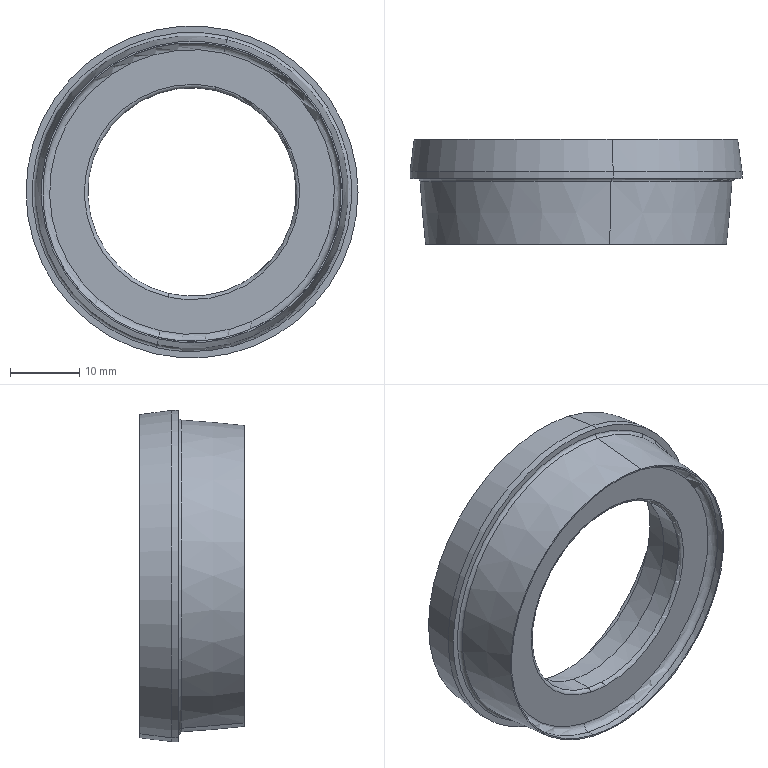Part | SolidWorks | features BaseBody 1 | 1 solid | 37 faces | box 47.8 x 15.1 x 47.8 mm | volume 5914 mm3 | cylinder 12 | torus 12 | plane 7 | cone 6 | commonest cylinder face diameters 30 x2 30.43 x2 35 x2 43 x2 46 x2 47.8 x2
STEP:
#1=CARTESIAN_POINT('',(1958.149,-234.4,875.416));
#2=VERTEX_POINT('',#1);
#3=CARTESIAN_POINT('',(1947.851,-234.4,830.584));
#4=VERTEX_POINT('',#3);
#5=CARTESIAN_POINT('',(1953.,-234.4,853.));
#6=DIRECTION('',(0.,-1.,0.));
#7=DIRECTION('',(0.9746,0.,-0.2239));
#8=AXIS2_PLACEMENT_3D('',#5,#6,#7);
#9=CIRCLE('',#8,23.);
#10=EDGE_CURVE('',#2,#4,#9,.T.);
#11=ORIENTED_EDGE('',*,*,#10,.T.);
#12=CARTESIAN_POINT('',(1947.851,-230.8,830.584));
#13=VERTEX_POINT('',#12);
#14=CARTESIAN_POINT('',(1947.851,-230.045,830.584));
#15=DIRECTION('',(0.,-1.,0.));
#16=VECTOR('',#15,1000.);
#17=LINE('',#14,#16);
#18=EDGE_CURVE('',#13,#4,#17,.T.);
#19=ORIENTED_EDGE('',*,*,#18,.F.);
#20=CARTESIAN_POINT('',(1958.149,-230.8,875.416));
#21=VERTEX_POINT('',#20);
#22=CARTESIAN_POINT('',(1953.,-230.8,853.));
#23=DIRECTION('',(0.,-1.,0.));
#24=DIRECTION('',(0.9746,0.,-0.2239));
#25=AXIS2_PLACEMENT_3D('',#22,#23,#24);
#26=CIRCLE('',#25,23.);
#27=EDGE_CURVE('',#21,#13,#26,.T.);
#28=ORIENTED_EDGE('',*,*,#27,.F.);
#29=CARTESIAN_POINT('',(1958.149,-230.045,875.416));
#30=DIRECTION('',(0.,1.,0.));
#31=VECTOR('',#30,1000.);
#32=LINE('',#29,#31);
#33=EDGE_CURVE('',#2,#21,#32,.T.);
#34=ORIENTED_EDGE('',*,*,#33,.F.);
#35=EDGE_LOOP('',(#11,#19,#28,#34));
#36=FACE_OUTER_BOUND('',#35,.T.);
#37=CARTESIAN_POINT('',(1953.,-230.045,853.));
#38=DIRECTION('',(0.,-1.,0.));
#39=DIRECTION('',(-0.2239,0.,-0.9746));
#40=AXIS2_PLACEMENT_3D('',#37,#38,#39);
#41=CYLINDRICAL_SURFACE('',#40,23.);
#42=ADVANCED_FACE('',(#36),#41,.F.);
#43=CARTESIAN_POINT('',(1957.701,-236.4,873.467));
#44=VERTEX_POINT('',#43);
#45=CARTESIAN_POINT('',(1948.299,-236.4,832.533));
#46=VERTEX_POINT('',#45);
#47=CARTESIAN_POINT('',(1953.,-236.4,853.));
#48=DIRECTION('',(0.,-1.,0.));
#49=DIRECTION('',(0.9746,0.,-0.2239));
#50=AXIS2_PLACEMENT_3D('',#47,#48,#49);
#51=CIRCLE('',#50,21.);
#52=EDGE_CURVE('',#44,#46,#51,.T.);
#53=ORIENTED_EDGE('',*,*,#52,.T.);
#54=CARTESIAN_POINT('',(1948.299,-234.4,832.533));
#55=DIRECTION('',(-0.9746,0.,0.2239));
#56=DIRECTION('',(0.,-1.,0.));
#57=AXIS2_PLACEMENT_3D('',#54,#55,#56);
#58=CIRCLE('',#57,2.);
#59=EDGE_CURVE('',#4,#46,#58,.T.);
#60=ORIENTED_EDGE('',*,*,#59,.F.);
#61=ORIENTED_EDGE('',*,*,#10,.F.);
#62=CARTESIAN_POINT('',(1957.701,-234.4,873.467));
#63=DIRECTION('',(-0.9746,0.,0.2239));
#64=DIRECTION('',(0.,-1.,0.));
#65=AXIS2_PLACEMENT_3D('',#62,#63,#64);
#66=CIRCLE('',#65,2.);
#67=EDGE_CURVE('',#44,#2,#66,.T.);
#68=ORIENTED_EDGE('',*,*,#67,.F.);
#69=EDGE_LOOP('',(#53,#60,#61,#68));
#70=FACE_OUTER_BOUND('',#69,.T.);
#71=CARTESIAN_POINT('',(1953.,-234.4,853.));
#72=DIRECTION('',(0.,-1.,0.));
#73=DIRECTION('',(-0.2239,0.,-0.9746));
#74=AXIS2_PLACEMENT_3D('',#71,#72,#73);
#75=TOROIDAL_SURFACE('',#74,21.,2.);
#76=ADVANCED_FACE('',(#70),#75,.F.);
#77=CARTESIAN_POINT('',(1953.,-230.8,853.));
#78=DIRECTION('',(0.,1.,0.));
#79=DIRECTION('',(0.9746,0.,-0.2239));
#80=AXIS2_PLACEMENT_3D('',#77,#78,#79);
#81=CIRCLE('',#80,23.);
#82=EDGE_CURVE('',#21,#13,#81,.T.);
#83=ORIENTED_EDGE('',*,*,#82,.T.);
#84=ORIENTED_EDGE('',*,*,#18,.T.);
#85=CARTESIAN_POINT('',(1953.,-234.4,853.));
#86=DIRECTION('',(0.,1.,0.));
#87=DIRECTION('',(0.9746,0.,-0.2239));
#88=AXIS2_PLACEMENT_3D('',#85,#86,#87);
#89=CIRCLE('',#88,23.);
#90=EDGE_CURVE('',#2,#4,#89,.T.);
#91=ORIENTED_EDGE('',*,*,#90,.F.);
#92=ORIENTED_EDGE('',*,*,#33,.T.);
#93=EDGE_LOOP('',(#83,#84,#91,#92));
#94=FACE_OUTER_BOUND('',#93,.T.);
#95=CARTESIAN_POINT('',(1953.,-230.045,853.));
#96=DIRECTION('',(0.,-1.,0.));
#97=DIRECTION('',(0.2239,0.,0.9746));
#98=AXIS2_PLACEMENT_3D('',#95,#96,#97);
#99=CYLINDRICAL_SURFACE('',#98,23.);
#100=ADVANCED_FACE('',(#94),#99,.F.);
#101=CARTESIAN_POINT('',(1958.216,-230.8,875.709));
#102=VERTEX_POINT('',#101);
#103=CARTESIAN_POINT('',(1947.784,-230.8,830.291));
#104=VERTEX_POINT('',#103);
#105=CARTESIAN_POINT('',(1953.,-230.8,853.));
#106=DIRECTION('',(0.,-1.,0.));
#107=DIRECTION('',(0.9746,0.,-0.2239));
#108=AXIS2_PLACEMENT_3D('',#105,#106,#107);
#109=CIRCLE('',#108,23.3);
#110=EDGE_CURVE('',#102,#104,#109,.T.);
#111=ORIENTED_EDGE('',*,*,#110,.F.);
#112=CARTESIAN_POINT('',(1958.216,-230.8,875.709));
#113=CARTESIAN_POINT('',(1960.29,-230.8,875.232));
#114=CARTESIAN_POINT('',(1962.31,-230.8,874.519));
#115=CARTESIAN_POINT('',(1964.24,-230.8,873.577));
#116=CARTESIAN_POINT('',(1967.849,-230.8,871.269));
#117=CARTESIAN_POINT('',(1970.846,-230.8,868.208));
#118=CARTESIAN_POINT('',(1972.162,-230.8,866.511));
#119=CARTESIAN_POINT('',(1974.384,-230.8,862.849));
#120=CARTESIAN_POINT('',(1975.723,-230.8,858.779));
#121=CARTESIAN_POINT('',(1976.157,-230.8,856.676));
#122=CARTESIAN_POINT('',(1976.536,-230.8,852.409));
#123=CARTESIAN_POINT('',(1975.943,-230.8,848.166));
#124=CARTESIAN_POINT('',(1975.404,-230.8,846.087));
#125=CARTESIAN_POINT('',(1973.863,-230.8,842.09));
#126=CARTESIAN_POINT('',(1971.46,-230.8,838.544));
#127=CARTESIAN_POINT('',(1970.06,-230.8,836.916));
#128=CARTESIAN_POINT('',(1966.913,-230.8,834.008));
#129=CARTESIAN_POINT('',(1963.192,-230.8,831.885));
#130=CARTESIAN_POINT('',(1961.218,-230.8,831.041));
#131=CARTESIAN_POINT('',(1957.361,-230.8,829.893));
#132=CARTESIAN_POINT('',(1953.354,-230.8,829.59));
#133=CARTESIAN_POINT('',(1951.471,-230.8,829.637));
#134=CARTESIAN_POINT('',(1949.607,-230.8,829.873));
#135=CARTESIAN_POINT('',(1947.784,-230.8,830.291));
#136=B_SPLINE_CURVE_WITH_KNOTS('',5,(#112,#113,#114,#115,#116,#117,#118,#119,#120,#121,#122,#123,#124,#125,#126,#127,#128,#129,#130,#131,#132,#133,#134,#135),.UNSPECIFIED.,.F.,.F.,(6,3,3,3,3,3,3,6),(0.,0.1454,0.2908,0.4361,0.5815,0.7269,0.8723,1.),.UNSPECIFIED.);
#137=EDGE_CURVE('',#102,#104,#136,.T.);
#138=ORIENTED_EDGE('',*,*,#137,.T.);
#139=EDGE_LOOP('',(#111,#138));
#140=FACE_OUTER_BOUND('',#139,.T.);
#141=ORIENTED_EDGE('',*,*,#82,.F.);
#142=ORIENTED_EDGE('',*,*,#27,.T.);
#143=EDGE_LOOP('',(#141,#142));
#144=FACE_BOUND('',#143,.T.);
#145=CARTESIAN_POINT('',(1953.,-230.8,853.));
#146=DIRECTION('',(0.,-1.,0.));
#147=DIRECTION('',(0.2239,0.,0.9746));
#148=AXIS2_PLACEMENT_3D('',#145,#146,#147);
#149=PLANE('',#148);
#150=ADVANCED_FACE('',(#140,#144),#149,.F.);
#151=ORIENTED_EDGE('',*,*,#52,.F.);
#152=CARTESIAN_POINT('',(1957.701,-236.4,873.467));
#153=CARTESIAN_POINT('',(1959.67,-236.4,873.015));
#154=CARTESIAN_POINT('',(1961.585,-236.4,872.326));
#155=CARTESIAN_POINT('',(1963.408,-236.4,871.408));
#156=CARTESIAN_POINT('',(1966.796,-236.4,869.153));
#157=CARTESIAN_POINT('',(1969.553,-236.4,866.159));
#158=CARTESIAN_POINT('',(1970.744,-236.4,864.503));
#159=CARTESIAN_POINT('',(1972.705,-236.4,860.936));
#160=CARTESIAN_POINT('',(1973.764,-236.4,857.006));
#161=CARTESIAN_POINT('',(1974.053,-236.4,854.987));
#162=CARTESIAN_POINT('',(1974.141,-236.4,850.917));
#163=CARTESIAN_POINT('',(1973.261,-236.4,846.944));
#164=CARTESIAN_POINT('',(1972.583,-236.4,845.019));
#165=CARTESIAN_POINT('',(1970.778,-236.4,841.371));
#166=CARTESIAN_POINT('',(1968.159,-236.4,838.256));
#167=CARTESIAN_POINT('',(1966.667,-236.4,836.863));
#168=CARTESIAN_POINT('',(1963.379,-236.4,834.465));
#169=CARTESIAN_POINT('',(1959.616,-236.4,832.915));
#170=CARTESIAN_POINT('',(1957.649,-236.4,832.371));
#171=CARTESIAN_POINT('',(1954.569,-236.4,831.908));
#172=CARTESIAN_POINT('',(1951.473,-236.4,832.014));
#173=CARTESIAN_POINT('',(1950.403,-236.4,832.12));
#174=CARTESIAN_POINT('',(1949.343,-236.4,832.293));
#175=CARTESIAN_POINT('',(1948.299,-236.4,832.533));
#176=B_SPLINE_CURVE_WITH_KNOTS('',5,(#152,#153,#154,#155,#156,#157,#158,#159,#160,#161,#162,#163,#164,#165,#166,#167,#168,#169,#170,#171,#172,#173,#174,#175),.UNSPECIFIED.,.F.,.F.,(6,3,3,3,3,3,3,6),(0.,0.1531,0.3063,0.4594,0.6125,0.7656,0.9188,1.),.UNSPECIFIED.);
#177=EDGE_CURVE('',#44,#46,#176,.T.);
#178=ORIENTED_EDGE('',*,*,#177,.T.);
#179=EDGE_LOOP('',(#151,#178));
#180=FACE_OUTER_BOUND('',#179,.T.);
#181=CARTESIAN_POINT('',(1957.03,-236.4,870.543));
#182=VERTEX_POINT('',#181);
#183=CARTESIAN_POINT('',(1948.97,-236.4,835.457));
#184=VERTEX_POINT('',#183);
#185=CARTESIAN_POINT('',(1957.03,-236.4,870.543));
#186=CARTESIAN_POINT('',(1958.65,-236.4,870.171));
#187=CARTESIAN_POINT('',(1960.228,-236.4,869.612));
#188=CARTESIAN_POINT('',(1961.734,-236.4,868.872));
#189=CARTESIAN_POINT('',(1964.547,-236.4,867.058));
#190=CARTESIAN_POINT('',(1966.873,-236.4,864.65));
#191=CARTESIAN_POINT('',(1967.891,-236.4,863.317));
#192=CARTESIAN_POINT('',(1969.602,-236.4,860.439));
#193=CARTESIAN_POINT('',(1970.611,-236.4,857.247));
#194=CARTESIAN_POINT('',(1970.928,-236.4,855.6));
#195=CARTESIAN_POINT('',(1971.177,-236.4,852.261));
#196=CARTESIAN_POINT('',(1970.658,-236.4,848.954));
#197=CARTESIAN_POINT('',(1970.208,-236.4,847.338));
#198=CARTESIAN_POINT('',(1968.943,-236.4,844.238));
#199=CARTESIAN_POINT('',(1967.005,-236.4,841.509));
#200=CARTESIAN_POINT('',(1965.882,-236.4,840.262));
#201=CARTESIAN_POINT('',(1963.368,-236.4,838.052));
#202=CARTESIAN_POINT('',(1960.417,-236.4,836.472));
#203=CARTESIAN_POINT('',(1958.856,-236.4,835.857));
#204=CARTESIAN_POINT('',(1955.941,-236.4,835.083));
#205=CARTESIAN_POINT('',(1952.936,-236.4,834.926));
#206=CARTESIAN_POINT('',(1951.597,-236.4,834.98));
#207=CARTESIAN_POINT('',(1950.27,-236.4,835.158));
#208=CARTESIAN_POINT('',(1948.97,-236.4,835.457));
#209=B_SPLINE_CURVE_WITH_KNOTS('',5,(#185,#186,#187,#188,#189,#190,#191,#192,#193,#194,#195,#196,#197,#198,#199,#200,#201,#202,#203,#204,#205,#206,#207,#208),.UNSPECIFIED.,.F.,.F.,(6,3,3,3,3,3,3,6),(0.,0.147,0.294,0.4411,0.5881,0.7351,0.8821,1.),.UNSPECIFIED.);
#210=EDGE_CURVE('',#182,#184,#209,.T.);
#211=ORIENTED_EDGE('',*,*,#210,.F.);
#212=CARTESIAN_POINT('',(1953.,-236.4,853.));
#213=DIRECTION('',(0.,-1.,0.));
#214=DIRECTION('',(0.9746,0.,-0.2239));
#215=AXIS2_PLACEMENT_3D('',#212,#213,#214);
#216=CIRCLE('',#215,18.);
#217=EDGE_CURVE('',#182,#184,#216,.T.);
#218=ORIENTED_EDGE('',*,*,#217,.T.);
#219=EDGE_LOOP('',(#211,#218));
#220=FACE_BOUND('',#219,.T.);
#221=CARTESIAN_POINT('',(1953.,-236.4,853.));
#222=DIRECTION('',(0.,-1.,0.));
#223=DIRECTION('',(0.2239,0.,0.9746));
#224=AXIS2_PLACEMENT_3D('',#221,#222,#223);
#225=PLANE('',#224);
#226=ADVANCED_FACE('',(#180,#220),#225,.F.);
#227=ORIENTED_EDGE('',*,*,#90,.T.);
#228=ORIENTED_EDGE('',*,*,#59,.T.);
#229=ORIENTED_EDGE('',*,*,#177,.F.);
#230=ORIENTED_EDGE('',*,*,#67,.T.);
#231=EDGE_LOOP('',(#227,#228,#229,#230));
#232=FACE_OUTER_BOUND('',#231,.T.);
#233=CARTESIAN_POINT('',(1953.,-234.4,853.));
#234=DIRECTION('',(0.,-1.,0.));
#235=DIRECTION('',(0.2239,0.,0.9746));
#236=AXIS2_PLACEMENT_3D('',#233,#234,#235);
#237=TOROIDAL_SURFACE('',#236,21.,2.);
#238=ADVANCED_FACE('',(#232),#237,.F.);
#239=ORIENTED_EDGE('',*,*,#110,.T.);
#240=CARTESIAN_POINT('',(1947.65,-235.4,829.707));
#241=VERTEX_POINT('',#240);
#242=CARTESIAN_POINT('',(-12527.07,-495942.839,-62186.75));
#243=DIRECTION('',(0.02895,0.9916,0.1261));
#244=VECTOR('',#243,1000.);
#245=LINE('',#242,#244);
#246=EDGE_CURVE('',#241,#104,#245,.T.);
#247=ORIENTED_EDGE('',*,*,#246,.F.);
#248=CARTESIAN_POINT('',(1958.35,-235.4,876.293));
#249=VERTEX_POINT('',#248);
#250=CARTESIAN_POINT('',(1953.,-235.4,853.));
#251=DIRECTION('',(0.,-1.,0.));
#252=DIRECTION('',(0.9746,0.,-0.2239));
#253=AXIS2_PLACEMENT_3D('',#250,#251,#252);
#254=CIRCLE('',#253,23.9);
#255=EDGE_CURVE('',#249,#241,#254,.T.);
#256=ORIENTED_EDGE('',*,*,#255,.F.);
#257=CARTESIAN_POINT('',(16433.07,-495942.839,63892.75));
#258=DIRECTION('',(0.02895,-0.9916,0.1261));
#259=VECTOR('',#258,1000.);
#260=LINE('',#257,#259);
#261=EDGE_CURVE('',#102,#249,#260,.T.);
#262=ORIENTED_EDGE('',*,*,#261,.F.);
#263=EDGE_LOOP('',(#239,#247,#256,#262));
#264=FACE_OUTER_BOUND('',#263,.T.);
#265=CARTESIAN_POINT('',(1953.,-233.1,853.));
#266=DIRECTION('',(0.,-1.,0.));
#267=DIRECTION('',(-0.2239,0.,-0.9746));
#268=AXIS2_PLACEMENT_3D('',#265,#266,#267);
#269=CONICAL_SURFACE('',#268,23.6,0.1297);
#270=ADVANCED_FACE('',(#264),#269,.T.);
#271=CARTESIAN_POINT('',(1953.,-235.4,853.));
#272=DIRECTION('',(0.,1.,0.));
#273=DIRECTION('',(0.9746,0.,-0.2239));
#274=AXIS2_PLACEMENT_3D('',#271,#272,#273);
#275=CIRCLE('',#274,23.9);
#276=EDGE_CURVE('',#249,#241,#275,.T.);
#277=ORIENTED_EDGE('',*,*,#276,.T.);
#278=ORIENTED_EDGE('',*,*,#246,.T.);
#279=ORIENTED_EDGE('',*,*,#137,.F.);
#280=ORIENTED_EDGE('',*,*,#261,.T.);
#281=EDGE_LOOP('',(#277,#278,#279,#280));
#282=FACE_OUTER_BOUND('',#281,.T.);
#283=CARTESIAN_POINT('',(1953.,-233.1,853.));
#284=DIRECTION('',(0.,-1.,0.));
#285=DIRECTION('',(0.2239,0.,0.9746));
#286=AXIS2_PLACEMENT_3D('',#283,#284,#285);
#287=CONICAL_SURFACE('',#286,23.6,0.1297);
#288=ADVANCED_FACE('',(#282),#287,.T.);
#289=ORIENTED_EDGE('',*,*,#210,.T.);
#290=CARTESIAN_POINT('',(1949.082,-235.9,835.944));
#291=VERTEX_POINT('',#290);
#292=CARTESIAN_POINT('',(1948.97,-235.9,835.457));
#293=DIRECTION('',(0.9746,0.,-0.2239));
#294=DIRECTION('',(0.,-1.,0.));
#295=AXIS2_PLACEMENT_3D('',#292,#293,#294);
#296=CIRCLE('',#295,0.5);
#297=EDGE_CURVE('',#291,#184,#296,.T.);
#298=ORIENTED_EDGE('',*,*,#297,.F.);
#299=CARTESIAN_POINT('',(1956.918,-235.9,870.056));
#300=VERTEX_POINT('',#299);
#301=CARTESIAN_POINT('',(1953.,-235.9,853.));
#302=DIRECTION('',(0.,1.,0.));
#303=DIRECTION('',(0.9746,0.,-0.2239));
#304=AXIS2_PLACEMENT_3D('',#301,#302,#303);
#305=CIRCLE('',#304,17.5);
#306=EDGE_CURVE('',#300,#291,#305,.T.);
#307=ORIENTED_EDGE('',*,*,#306,.F.);
#308=CARTESIAN_POINT('',(1957.03,-235.9,870.543));
#309=DIRECTION('',(0.9746,0.,-0.2239));
#310=DIRECTION('',(0.,-1.,0.));
#311=AXIS2_PLACEMENT_3D('',#308,#309,#310);
#312=CIRCLE('',#311,0.5);
#313=EDGE_CURVE('',#182,#300,#312,.T.);
#314=ORIENTED_EDGE('',*,*,#313,.F.);
#315=EDGE_LOOP('',(#289,#298,#307,#314));
#316=FACE_OUTER_BOUND('',#315,.T.);
#317=CARTESIAN_POINT('',(1953.,-235.9,853.));
#318=DIRECTION('',(0.,-1.,0.));
#319=DIRECTION('',(0.2239,0.,0.9746));
#320=AXIS2_PLACEMENT_3D('',#317,#318,#319);
#321=TOROIDAL_SURFACE('',#320,18.,0.5);
#322=ADVANCED_FACE('',(#316),#321,.F.);
#323=CARTESIAN_POINT('',(1953.,-235.9,853.));
#324=DIRECTION('',(0.,-1.,0.));
#325=DIRECTION('',(0.9746,0.,-0.2239));
#326=AXIS2_PLACEMENT_3D('',#323,#324,#325);
#327=CIRCLE('',#326,17.5);
#328=EDGE_CURVE('',#300,#291,#327,.T.);
#329=ORIENTED_EDGE('',*,*,#328,.T.);
#330=ORIENTED_EDGE('',*,*,#297,.T.);
#331=ORIENTED_EDGE('',*,*,#217,.F.);
#332=ORIENTED_EDGE('',*,*,#313,.T.);
#333=EDGE_LOOP('',(#329,#330,#331,#332));
#334=FACE_OUTER_BOUND('',#333,.T.);
#335=CARTESIAN_POINT('',(1953.,-235.9,853.));
#336=DIRECTION('',(0.,-1.,0.));
#337=DIRECTION('',(-0.2239,0.,-0.9746));
#338=AXIS2_PLACEMENT_3D('',#335,#336,#337);
#339=TOROIDAL_SURFACE('',#338,18.,0.5);
#340=ADVANCED_FACE('',(#334),#339,.F.);
#341=ORIENTED_EDGE('',*,*,#255,.T.);
#342=CARTESIAN_POINT('',(1947.65,-236.4,829.707));
#343=VERTEX_POINT('',#342);
#344=CARTESIAN_POINT('',(1947.65,-230.045,829.707));
#345=DIRECTION('',(0.,-1.,0.));
#346=VECTOR('',#345,1000.);
#347=LINE('',#344,#346);
#348=EDGE_CURVE('',#241,#343,#347,.T.);
#349=ORIENTED_EDGE('',*,*,#348,.T.);
#350=CARTESIAN_POINT('',(1958.35,-236.4,876.293));
#351=VERTEX_POINT('',#350);
#352=CARTESIAN_POINT('',(1953.,-236.4,853.));
#353=DIRECTION('',(0.,-1.,0.));
#354=DIRECTION('',(0.9746,0.,-0.2239));
#355=AXIS2_PLACEMENT_3D('',#352,#353,#354);
#356=CIRCLE('',#355,23.9);
#357=EDGE_CURVE('',#351,#343,#356,.T.);
#358=ORIENTED_EDGE('',*,*,#357,.F.);
#359=CARTESIAN_POINT('',(1958.35,-230.045,876.293));
#360=DIRECTION('',(0.,1.,0.));
#361=VECTOR('',#360,1000.);
#362=LINE('',#359,#361);
#363=EDGE_CURVE('',#351,#249,#362,.T.);
#364=ORIENTED_EDGE('',*,*,#363,.T.);
#365=EDGE_LOOP('',(#341,#349,#358,#364));
#366=FACE_OUTER_BOUND('',#365,.T.);
#367=CARTESIAN_POINT('',(1953.,-230.045,853.));
#368=DIRECTION('',(0.,-1.,0.));
#369=DIRECTION('',(-0.2239,0.,-0.9746));
#370=AXIS2_PLACEMENT_3D('',#367,#368,#369);
#371=CYLINDRICAL_SURFACE('',#370,23.9);
#372=ADVANCED_FACE('',(#366),#371,.T.);
#373=CARTESIAN_POINT('',(1953.,-236.4,853.));
#374=DIRECTION('',(0.,1.,0.));
#375=DIRECTION('',(0.9746,0.,-0.2239));
#376=AXIS2_PLACEMENT_3D('',#373,#374,#375);
#377=CIRCLE('',#376,23.9);
#378=EDGE_CURVE('',#351,#343,#377,.T.);
#379=ORIENTED_EDGE('',*,*,#378,.T.);
#380=ORIENTED_EDGE('',*,*,#348,.F.);
#381=ORIENTED_EDGE('',*,*,#276,.F.);
#382=ORIENTED_EDGE('',*,*,#363,.F.);
#383=EDGE_LOOP('',(#379,#380,#381,#382));
#384=FACE_OUTER_BOUND('',#383,.T.);
#385=CARTESIAN_POINT('',(1953.,-230.045,853.));
#386=DIRECTION('',(0.,-1.,0.));
#387=DIRECTION('',(0.2239,0.,0.9746));
#388=AXIS2_PLACEMENT_3D('',#385,#386,#387);
#389=CYLINDRICAL_SURFACE('',#388,23.9);
#390=ADVANCED_FACE('',(#384),#389,.T.);
#391=ORIENTED_EDGE('',*,*,#306,.T.);
#392=CARTESIAN_POINT('',(1949.082,-235.4,835.944));
#393=VERTEX_POINT('',#392);
#394=CARTESIAN_POINT('',(1949.082,-230.045,835.944));
#395=DIRECTION('',(0.,1.,0.));
#396=VECTOR('',#395,1000.);
#397=LINE('',#394,#396);
#398=EDGE_CURVE('',#291,#393,#397,.T.);
#399=ORIENTED_EDGE('',*,*,#398,.T.);
#400=CARTESIAN_POINT('',(1956.918,-235.4,870.056));
#401=VERTEX_POINT('',#400);
#402=CARTESIAN_POINT('',(1953.,-235.4,853.));
#403=DIRECTION('',(0.,1.,0.));
#404=DIRECTION('',(0.9746,0.,-0.2239));
#405=AXIS2_PLACEMENT_3D('',#402,#403,#404);
#406=CIRCLE('',#405,17.5);
#407=EDGE_CURVE('',#401,#393,#406,.T.);
#408=ORIENTED_EDGE('',*,*,#407,.F.);
#409=CARTESIAN_POINT('',(1956.918,-230.045,870.056));
#410=DIRECTION('',(0.,-1.,0.));
#411=VECTOR('',#410,1000.);
#412=LINE('',#409,#411);
#413=EDGE_CURVE('',#401,#300,#412,.T.);
#414=ORIENTED_EDGE('',*,*,#413,.T.);
#415=EDGE_LOOP('',(#391,#399,#408,#414));
#416=FACE_OUTER_BOUND('',#415,.T.);
#417=CARTESIAN_POINT('',(1953.,-230.045,853.));
#418=DIRECTION('',(0.,-1.,0.));
#419=DIRECTION('',(0.2239,0.,0.9746));
#420=AXIS2_PLACEMENT_3D('',#417,#418,#419);
#421=CYLINDRICAL_SURFACE('',#420,17.5);
#422=ADVANCED_FACE('',(#416),#421,.T.);
#423=CARTESIAN_POINT('',(1953.,-235.4,853.));
#424=DIRECTION('',(0.,-1.,0.));
#425=DIRECTION('',(0.9746,0.,-0.2239));
#426=AXIS2_PLACEMENT_3D('',#423,#424,#425);
#427=CIRCLE('',#426,17.5);
#428=EDGE_CURVE('',#401,#393,#427,.T.);
#429=ORIENTED_EDGE('',*,*,#428,.T.);
#430=ORIENTED_EDGE('',*,*,#398,.F.);
#431=ORIENTED_EDGE('',*,*,#328,.F.);
#432=ORIENTED_EDGE('',*,*,#413,.F.);
#433=EDGE_LOOP('',(#429,#430,#431,#432));
#434=FACE_OUTER_BOUND('',#433,.T.);
#435=CARTESIAN_POINT('',(1953.,-230.045,853.));
#436=DIRECTION('',(0.,-1.,0.));
#437=DIRECTION('',(-0.2239,0.,-0.9746));
#438=AXIS2_PLACEMENT_3D('',#435,#436,#437);
#439=CYLINDRICAL_SURFACE('',#438,17.5);
#440=ADVANCED_FACE('',(#434),#439,.T.);
#441=ORIENTED_EDGE('',*,*,#378,.F.);
#442=ORIENTED_EDGE('',*,*,#357,.T.);
#443=EDGE_LOOP('',(#441,#442));
#444=FACE_OUTER_BOUND('',#443,.T.);
#445=CARTESIAN_POINT('',(1958.147,-236.4,875.406));
#446=VERTEX_POINT('',#445);
#447=CARTESIAN_POINT('',(1947.853,-236.4,830.594));
#448=VERTEX_POINT('',#447);
#449=CARTESIAN_POINT('',(1953.,-236.4,853.));
#450=DIRECTION('',(0.,-1.,0.));
#451=DIRECTION('',(0.9746,0.,-0.2239));
#452=AXIS2_PLACEMENT_3D('',#449,#450,#451);
#453=CIRCLE('',#452,22.989);
#454=EDGE_CURVE('',#446,#448,#453,.T.);
#455=ORIENTED_EDGE('',*,*,#454,.F.);
#456=CARTESIAN_POINT('',(1958.147,-236.4,875.406));
#457=CARTESIAN_POINT('',(1960.207,-236.4,874.933));
#458=CARTESIAN_POINT('',(1962.213,-236.4,874.222));
#459=CARTESIAN_POINT('',(1964.128,-236.4,873.284));
#460=CARTESIAN_POINT('',(1967.709,-236.4,870.983));
#461=CARTESIAN_POINT('',(1970.674,-236.4,867.93));
#462=CARTESIAN_POINT('',(1971.974,-236.4,866.239));
#463=CARTESIAN_POINT('',(1974.161,-236.4,862.589));
#464=CARTESIAN_POINT('',(1975.464,-236.4,858.537));
#465=CARTESIAN_POINT('',(1975.878,-236.4,856.445));
#466=CARTESIAN_POINT('',(1976.219,-236.4,852.202));
#467=CARTESIAN_POINT('',(1975.588,-236.4,847.993));
#468=CARTESIAN_POINT('',(1975.031,-236.4,845.935));
#469=CARTESIAN_POINT('',(1973.453,-236.4,841.982));
#470=CARTESIAN_POINT('',(1971.02,-236.4,838.49));
#471=CARTESIAN_POINT('',(1969.607,-236.4,836.892));
#472=CARTESIAN_POINT('',(1966.44,-236.4,834.05));
#473=CARTESIAN_POINT('',(1962.71,-236.4,832.));
#474=CARTESIAN_POINT('',(1960.735,-236.4,831.195));
#475=CARTESIAN_POINT('',(1956.978,-236.4,830.149));
#476=CARTESIAN_POINT('',(1953.093,-236.4,829.909));
#477=CARTESIAN_POINT('',(1951.323,-236.4,829.97));
#478=CARTESIAN_POINT('',(1949.569,-236.4,830.2));
#479=CARTESIAN_POINT('',(1947.853,-236.4,830.594));
#480=B_SPLINE_CURVE_WITH_KNOTS('',5,(#456,#457,#458,#459,#460,#461,#462,#463,#464,#465,#466,#467,#468,#469,#470,#471,#472,#473,#474,#475,#476,#477,#478,#479),.UNSPECIFIED.,.F.,.F.,(6,3,3,3,3,3,3,6),(0.,0.1464,0.2927,0.4391,0.5854,0.7318,0.8781,1.),.UNSPECIFIED.);
#481=EDGE_CURVE('',#446,#448,#480,.T.);
#482=ORIENTED_EDGE('',*,*,#481,.T.);
#483=EDGE_LOOP('',(#455,#482));
#484=FACE_BOUND('',#483,.T.);
#485=CARTESIAN_POINT('',(1953.,-236.4,853.));
#486=DIRECTION('',(0.,-1.,0.));
#487=DIRECTION('',(0.2239,0.,0.9746));
#488=AXIS2_PLACEMENT_3D('',#485,#486,#487);
#489=PLANE('',#488);
#490=ADVANCED_FACE('',(#444,#484),#489,.T.);
#491=ORIENTED_EDGE('',*,*,#428,.F.);
#492=ORIENTED_EDGE('',*,*,#407,.T.);
#493=EDGE_LOOP('',(#491,#492));
#494=FACE_OUTER_BOUND('',#493,.T.);
#495=CARTESIAN_POINT('',(1956.851,-235.4,869.763));
#496=VERTEX_POINT('',#495);
#497=CARTESIAN_POINT('',(1949.149,-235.4,836.237));
#498=VERTEX_POINT('',#497);
#499=CARTESIAN_POINT('',(1956.851,-235.4,869.763));
#500=CARTESIAN_POINT('',(1958.435,-235.4,869.4));
#501=CARTESIAN_POINT('',(1959.976,-235.4,868.849));
#502=CARTESIAN_POINT('',(1961.445,-235.4,868.117));
#503=CARTESIAN_POINT('',(1964.181,-235.4,866.321));
#504=CARTESIAN_POINT('',(1966.424,-235.4,863.937));
#505=CARTESIAN_POINT('',(1967.399,-235.4,862.618));
#506=CARTESIAN_POINT('',(1969.019,-235.4,859.773));
#507=CARTESIAN_POINT('',(1969.931,-235.4,856.629));
#508=CARTESIAN_POINT('',(1970.199,-235.4,855.011));
#509=CARTESIAN_POINT('',(1970.346,-235.4,851.74));
#510=CARTESIAN_POINT('',(1969.728,-235.4,848.526));
#511=CARTESIAN_POINT('',(1969.229,-235.4,846.963));
#512=CARTESIAN_POINT('',(1967.873,-235.4,843.984));
#513=CARTESIAN_POINT('',(1965.859,-235.4,841.403));
#514=CARTESIAN_POINT('',(1964.704,-235.4,840.238));
#515=CARTESIAN_POINT('',(1962.14,-235.4,838.203));
#516=CARTESIAN_POINT('',(1959.172,-235.4,836.821));
#517=CARTESIAN_POINT('',(1957.613,-235.4,836.31));
#518=CARTESIAN_POINT('',(1954.967,-235.4,835.778));
#519=CARTESIAN_POINT('',(1952.279,-235.4,835.766));
#520=CARTESIAN_POINT('',(1951.223,-235.4,835.843));
#521=CARTESIAN_POINT('',(1950.177,-235.4,836.));
#522=CARTESIAN_POINT('',(1949.149,-235.4,836.237));
#523=B_SPLINE_CURVE_WITH_KNOTS('',5,(#499,#500,#501,#502,#503,#504,#505,#506,#507,#508,#509,#510,#511,#512,#513,#514,#515,#516,#517,#518,#519,#520,#521,#522),.UNSPECIFIED.,.F.,.F.,(6,3,3,3,3,3,3,6),(0.,0.1504,0.3008,0.4512,0.6016,0.752,0.9024,1.),.UNSPECIFIED.);
#524=EDGE_CURVE('',#496,#498,#523,.T.);
#525=ORIENTED_EDGE('',*,*,#524,.F.);
#526=CARTESIAN_POINT('',(1953.,-235.4,853.));
#527=DIRECTION('',(0.,-1.,0.));
#528=DIRECTION('',(0.9746,0.,-0.2239));
#529=AXIS2_PLACEMENT_3D('',#526,#527,#528);
#530=CIRCLE('',#529,17.2);
#531=EDGE_CURVE('',#496,#498,#530,.T.);
#532=ORIENTED_EDGE('',*,*,#531,.T.);
#533=EDGE_LOOP('',(#525,#532));
#534=FACE_BOUND('',#533,.T.);
#535=CARTESIAN_POINT('',(1953.,-235.4,853.));
#536=DIRECTION('',(0.,-1.,0.));
#537=DIRECTION('',(0.2239,0.,0.9746));
#538=AXIS2_PLACEMENT_3D('',#535,#536,#537);
#539=PLANE('',#538);
#540=ADVANCED_FACE('',(#494,#534),#539,.F.);
#541=ORIENTED_EDGE('',*,*,#454,.T.);
#542=CARTESIAN_POINT('',(1947.965,-236.856,831.08));
#543=VERTEX_POINT('',#542);
#544=CARTESIAN_POINT('',(1947.853,-236.9,830.594));
#545=DIRECTION('',(0.9746,0.,-0.2239));
#546=DIRECTION('',(0.,-1.,0.));
#547=AXIS2_PLACEMENT_3D('',#544,#545,#546);
#548=CIRCLE('',#547,0.5);
#549=EDGE_CURVE('',#448,#543,#548,.T.);
#550=ORIENTED_EDGE('',*,*,#549,.T.);
#551=CARTESIAN_POINT('',(1958.035,-236.856,874.92));
#552=VERTEX_POINT('',#551);
#553=CARTESIAN_POINT('',(1953.,-236.856,853.));
#554=DIRECTION('',(0.,-1.,0.));
#555=DIRECTION('',(0.9746,0.,-0.2239));
#556=AXIS2_PLACEMENT_3D('',#553,#554,#555);
#557=CIRCLE('',#556,22.491);
#558=EDGE_CURVE('',#552,#543,#557,.T.);
#559=ORIENTED_EDGE('',*,*,#558,.F.);
#560=CARTESIAN_POINT('',(1958.147,-236.9,875.406));
#561=DIRECTION('',(0.9746,0.,-0.2239));
#562=DIRECTION('',(0.,-1.,0.));
#563=AXIS2_PLACEMENT_3D('',#560,#561,#562);
#564=CIRCLE('',#563,0.5);
#565=EDGE_CURVE('',#552,#446,#564,.T.);
#566=ORIENTED_EDGE('',*,*,#565,.T.);
#567=EDGE_LOOP('',(#541,#550,#559,#566));
#568=FACE_OUTER_BOUND('',#567,.T.);
#569=CARTESIAN_POINT('',(1953.,-236.9,853.));
#570=DIRECTION('',(0.,-1.,0.));
#571=DIRECTION('',(-0.2239,0.,-0.9746));
#572=AXIS2_PLACEMENT_3D('',#569,#570,#571);
#573=TOROIDAL_SURFACE('',#572,22.989,0.5);
#574=ADVANCED_FACE('',(#568),#573,.F.);
#575=CARTESIAN_POINT('',(1953.,-236.856,853.));
#576=DIRECTION('',(0.,1.,0.));
#577=DIRECTION('',(0.9746,0.,-0.2239));
#578=AXIS2_PLACEMENT_3D('',#575,#576,#577);
#579=CIRCLE('',#578,22.491);
#580=EDGE_CURVE('',#552,#543,#579,.T.);
#581=ORIENTED_EDGE('',*,*,#580,.T.);
#582=ORIENTED_EDGE('',*,*,#549,.F.);
#583=ORIENTED_EDGE('',*,*,#481,.F.);
#584=ORIENTED_EDGE('',*,*,#565,.F.);
#585=EDGE_LOOP('',(#581,#582,#583,#584));
#586=FACE_OUTER_BOUND('',#585,.T.);
#587=CARTESIAN_POINT('',(1953.,-236.9,853.));
#588=DIRECTION('',(0.,-1.,0.));
#589=DIRECTION('',(0.2239,0.,0.9746));
#590=AXIS2_PLACEMENT_3D('',#587,#588,#589);
#591=TOROIDAL_SURFACE('',#590,22.989,0.5);
#592=ADVANCED_FACE('',(#586),#591,.F.);
#593=ORIENTED_EDGE('',*,*,#524,.T.);
#594=CARTESIAN_POINT('',(1949.298,-242.996,836.884));
#595=VERTEX_POINT('',#594);
#596=CARTESIAN_POINT('',(-7804.563,497761.752,-41627.066));
#597=DIRECTION('',(-0.01951,0.9962,-0.08494));
#598=VECTOR('',#597,1000.);
#599=LINE('',#596,#598);
#600=EDGE_CURVE('',#595,#498,#599,.T.);
#601=ORIENTED_EDGE('',*,*,#600,.F.);
#602=CARTESIAN_POINT('',(1956.702,-242.996,869.116));
#603=VERTEX_POINT('',#602);
#604=CARTESIAN_POINT('',(1953.,-242.996,853.));
#605=DIRECTION('',(0.,1.,0.));
#606=DIRECTION('',(-0.9746,0.,0.2239));
#607=AXIS2_PLACEMENT_3D('',#604,#605,#606);
#608=CIRCLE('',#607,16.535);
#609=EDGE_CURVE('',#603,#595,#608,.T.);
#610=ORIENTED_EDGE('',*,*,#609,.F.);
#611=CARTESIAN_POINT('',(11710.563,497761.752,43333.066));
#612=DIRECTION('',(-0.01951,-0.9962,-0.08494));
#613=VECTOR('',#612,1000.);
#614=LINE('',#611,#613);
#615=EDGE_CURVE('',#496,#603,#614,.T.);
#616=ORIENTED_EDGE('',*,*,#615,.F.);
#617=EDGE_LOOP('',(#593,#601,#610,#616));
#618=FACE_OUTER_BOUND('',#617,.T.);
#619=CARTESIAN_POINT('',(1953.,-239.198,853.));
#620=DIRECTION('',(0.,1.,0.));
#621=DIRECTION('',(-0.2239,0.,-0.9746));
#622=AXIS2_PLACEMENT_3D('',#619,#620,#621);
#623=CONICAL_SURFACE('',#622,16.868,0.08727);
#624=ADVANCED_FACE('',(#618),#623,.F.);
#625=CARTESIAN_POINT('',(1953.,-242.996,853.));
#626=DIRECTION('',(0.,-1.,0.));
#627=DIRECTION('',(-0.9746,0.,0.2239));
#628=AXIS2_PLACEMENT_3D('',#625,#626,#627);
#629=CIRCLE('',#628,16.535);
#630=EDGE_CURVE('',#603,#595,#629,.T.);
#631=ORIENTED_EDGE('',*,*,#630,.T.);
#632=ORIENTED_EDGE('',*,*,#600,.T.);
#633=ORIENTED_EDGE('',*,*,#531,.F.);
#634=ORIENTED_EDGE('',*,*,#615,.T.);
#635=EDGE_LOOP('',(#631,#632,#633,#634));
#636=FACE_OUTER_BOUND('',#635,.T.);
#637=CARTESIAN_POINT('',(1953.,-239.198,853.));
#638=DIRECTION('',(0.,1.,0.));
#639=DIRECTION('',(0.2239,0.,0.9746));
#640=AXIS2_PLACEMENT_3D('',#637,#638,#639);
#641=CONICAL_SURFACE('',#640,16.868,0.08727);
#642=ADVANCED_FACE('',(#636),#641,.F.);
#643=ORIENTED_EDGE('',*,*,#558,.T.);
#644=CARTESIAN_POINT('',(1948.142,-245.9,831.851));
#645=VERTEX_POINT('',#644);
#646=CARTESIAN_POINT('',(-7805.148,497729.694,-41629.613));
#647=DIRECTION('',(-0.01951,0.9962,-0.08494));
#648=VECTOR('',#647,1000.);
#649=LINE('',#646,#648);
#650=EDGE_CURVE('',#645,#543,#649,.T.);
#651=ORIENTED_EDGE('',*,*,#650,.F.);
#652=CARTESIAN_POINT('',(1957.858,-245.9,874.149));
#653=VERTEX_POINT('',#652);
#654=CARTESIAN_POINT('',(1953.,-245.9,853.));
#655=DIRECTION('',(0.,-1.,0.));
#656=DIRECTION('',(-0.9746,0.,0.2239));
#657=AXIS2_PLACEMENT_3D('',#654,#655,#656);
#658=CIRCLE('',#657,21.7);
#659=EDGE_CURVE('',#653,#645,#658,.T.);
#660=ORIENTED_EDGE('',*,*,#659,.F.);
#661=CARTESIAN_POINT('',(11711.148,497729.694,43335.613));
#662=DIRECTION('',(-0.01951,-0.9962,-0.08494));
#663=VECTOR('',#662,1000.);
#664=LINE('',#661,#663);
#665=EDGE_CURVE('',#552,#653,#664,.T.);
#666=ORIENTED_EDGE('',*,*,#665,.F.);
#667=EDGE_LOOP('',(#643,#651,#660,#666));
#668=FACE_OUTER_BOUND('',#667,.T.);
#669=CARTESIAN_POINT('',(1953.,-241.378,853.));
#670=DIRECTION('',(0.,1.,0.));
#671=DIRECTION('',(0.2239,0.,0.9746));
#672=AXIS2_PLACEMENT_3D('',#669,#670,#671);
#673=CONICAL_SURFACE('',#672,22.096,0.08727);
#674=ADVANCED_FACE('',(#668),#673,.T.);
#675=CARTESIAN_POINT('',(1953.,-245.9,853.));
#676=DIRECTION('',(0.,1.,0.));
#677=DIRECTION('',(-0.9746,0.,0.2239));
#678=AXIS2_PLACEMENT_3D('',#675,#676,#677);
#679=CIRCLE('',#678,21.7);
#680=EDGE_CURVE('',#653,#645,#679,.T.);
#681=ORIENTED_EDGE('',*,*,#680,.T.);
#682=ORIENTED_EDGE('',*,*,#650,.T.);
#683=ORIENTED_EDGE('',*,*,#580,.F.);
#684=ORIENTED_EDGE('',*,*,#665,.T.);
#685=EDGE_LOOP('',(#681,#682,#683,#684));
#686=FACE_OUTER_BOUND('',#685,.T.);
#687=CARTESIAN_POINT('',(1953.,-241.378,853.));
#688=DIRECTION('',(0.,1.,0.));
#689=DIRECTION('',(-0.2239,0.,-0.9746));
#690=AXIS2_PLACEMENT_3D('',#687,#688,#689);
#691=CONICAL_SURFACE('',#690,22.096,0.08727);
#692=ADVANCED_FACE('',(#686),#691,.T.);
#693=ORIENTED_EDGE('',*,*,#609,.T.);
#694=CARTESIAN_POINT('',(1949.594,-242.939,838.171));
#695=VERTEX_POINT('',#694);
#696=CARTESIAN_POINT('',(1949.446,-242.939,837.526));
#697=DIRECTION('',(0.9746,0.,-0.2239));
#698=DIRECTION('',(0.,-1.,0.));
#699=AXIS2_PLACEMENT_3D('',#696,#697,#698);
#700=CIRCLE('',#699,0.6615);
#701=EDGE_CURVE('',#695,#595,#700,.T.);
#702=ORIENTED_EDGE('',*,*,#701,.F.);
#703=CARTESIAN_POINT('',(1956.406,-242.939,867.829));
#704=VERTEX_POINT('',#703);
#705=CARTESIAN_POINT('',(1953.,-242.939,853.));
#706=DIRECTION('',(0.,1.,0.));
#707=DIRECTION('',(0.9746,0.,-0.2239));
#708=AXIS2_PLACEMENT_3D('',#705,#706,#707);
#709=CIRCLE('',#708,15.215);
#710=EDGE_CURVE('',#704,#695,#709,.T.);
#711=ORIENTED_EDGE('',*,*,#710,.F.);
#712=CARTESIAN_POINT('',(1956.554,-242.939,868.474));
#713=DIRECTION('',(0.9746,0.,-0.2239));
#714=DIRECTION('',(0.,-1.,0.));
#715=AXIS2_PLACEMENT_3D('',#712,#713,#714);
#716=CIRCLE('',#715,0.6615);
#717=EDGE_CURVE('',#603,#704,#716,.T.);
#718=ORIENTED_EDGE('',*,*,#717,.F.);
#719=EDGE_LOOP('',(#693,#702,#711,#718));
#720=FACE_OUTER_BOUND('',#719,.T.);
#721=CARTESIAN_POINT('',(1953.,-242.939,853.));
#722=DIRECTION('',(0.,-1.,0.));
#723=DIRECTION('',(0.2239,0.,0.9746));
#724=AXIS2_PLACEMENT_3D('',#721,#722,#723);
#725=TOROIDAL_SURFACE('',#724,15.876,0.6615);
#726=ADVANCED_FACE('',(#720),#725,.F.);
#727=CARTESIAN_POINT('',(1953.,-242.939,853.));
#728=DIRECTION('',(0.,-1.,0.));
#729=DIRECTION('',(0.9746,0.,-0.2239));
#730=AXIS2_PLACEMENT_3D('',#727,#728,#729);
#731=CIRCLE('',#730,15.215);
#732=EDGE_CURVE('',#704,#695,#731,.T.);
#733=ORIENTED_EDGE('',*,*,#732,.T.);
#734=ORIENTED_EDGE('',*,*,#701,.T.);
#735=ORIENTED_EDGE('',*,*,#630,.F.);
#736=ORIENTED_EDGE('',*,*,#717,.T.);
#737=EDGE_LOOP('',(#733,#734,#735,#736));
#738=FACE_OUTER_BOUND('',#737,.T.);
#739=CARTESIAN_POINT('',(1953.,-242.939,853.));
#740=DIRECTION('',(0.,-1.,0.));
#741=DIRECTION('',(-0.2239,0.,-0.9746));
#742=AXIS2_PLACEMENT_3D('',#739,#740,#741);
#743=TOROIDAL_SURFACE('',#742,15.876,0.6615);
#744=ADVANCED_FACE('',(#738),#743,.F.);
#745=ORIENTED_EDGE('',*,*,#680,.F.);
#746=ORIENTED_EDGE('',*,*,#659,.T.);
#747=EDGE_LOOP('',(#745,#746));
#748=FACE_OUTER_BOUND('',#747,.T.);
#749=CARTESIAN_POINT('',(1957.813,-245.9,873.954));
#750=VERTEX_POINT('',#749);
#751=CARTESIAN_POINT('',(1948.187,-245.9,832.046));
#752=VERTEX_POINT('',#751);
#753=CARTESIAN_POINT('',(1953.,-245.9,853.));
#754=DIRECTION('',(0.,-1.,0.));
#755=DIRECTION('',(0.9746,0.,-0.2239));
#756=AXIS2_PLACEMENT_3D('',#753,#754,#755);
#757=CIRCLE('',#756,21.5);
#758=EDGE_CURVE('',#750,#752,#757,.T.);
#759=ORIENTED_EDGE('',*,*,#758,.F.);
#760=CARTESIAN_POINT('',(1957.813,-245.9,873.954));
#761=CARTESIAN_POINT('',(1959.806,-245.9,873.497));
#762=CARTESIAN_POINT('',(1961.744,-245.9,872.802));
#763=CARTESIAN_POINT('',(1963.59,-245.9,871.879));
#764=CARTESIAN_POINT('',(1967.028,-245.9,869.613));
#765=CARTESIAN_POINT('',(1969.838,-245.9,866.604));
#766=CARTESIAN_POINT('',(1971.057,-245.9,864.938));
#767=CARTESIAN_POINT('',(1973.076,-245.9,861.349));
#768=CARTESIAN_POINT('',(1974.197,-245.9,857.387));
#769=CARTESIAN_POINT('',(1974.519,-245.9,855.349));
#770=CARTESIAN_POINT('',(1974.671,-245.9,851.234));
#771=CARTESIAN_POINT('',(1973.855,-245.9,847.198));
#772=CARTESIAN_POINT('',(1973.207,-245.9,845.238));
#773=CARTESIAN_POINT('',(1971.459,-245.9,841.51));
#774=CARTESIAN_POINT('',(1968.886,-245.9,838.296));
#775=CARTESIAN_POINT('',(1967.413,-245.9,836.85));
#776=CARTESIAN_POINT('',(1964.153,-245.9,834.335));
#777=CARTESIAN_POINT('',(1960.393,-245.9,832.655));
#778=CARTESIAN_POINT('',(1958.422,-245.9,832.043));
#779=CARTESIAN_POINT('',(1955.167,-245.9,831.446));
#780=CARTESIAN_POINT('',(1951.871,-245.9,831.476));
#781=CARTESIAN_POINT('',(1950.629,-245.9,831.577));
#782=CARTESIAN_POINT('',(1949.398,-245.9,831.768));
#783=CARTESIAN_POINT('',(1948.187,-245.9,832.046));
#784=B_SPLINE_CURVE_WITH_KNOTS('',5,(#760,#761,#762,#763,#764,#765,#766,#767,#768,#769,#770,#771,#772,#773,#774,#775,#776,#777,#778,#779,#780,#781,#782,#783),.UNSPECIFIED.,.F.,.F.,(6,3,3,3,3,3,3,6),(0.,0.1513,0.3027,0.454,0.6054,0.7567,0.908,1.),.UNSPECIFIED.);
#785=EDGE_CURVE('',#750,#752,#784,.T.);
#786=ORIENTED_EDGE('',*,*,#785,.T.);
#787=EDGE_LOOP('',(#759,#786));
#788=FACE_BOUND('',#787,.T.);
#789=CARTESIAN_POINT('',(1953.,-245.9,853.));
#790=DIRECTION('',(0.,-1.,0.));
#791=DIRECTION('',(0.2239,0.,0.9746));
#792=AXIS2_PLACEMENT_3D('',#789,#790,#791);
#793=PLANE('',#792);
#794=ADVANCED_FACE('',(#748,#788),#793,.T.);
#795=ORIENTED_EDGE('',*,*,#710,.T.);
#796=CARTESIAN_POINT('',(1949.594,-240.4,838.171));
#797=VERTEX_POINT('',#796);
#798=CARTESIAN_POINT('',(1949.594,-230.045,838.171));
#799=DIRECTION('',(0.,-1.,0.));
#800=VECTOR('',#799,1000.);
#801=LINE('',#798,#800);
#802=EDGE_CURVE('',#797,#695,#801,.T.);
#803=ORIENTED_EDGE('',*,*,#802,.F.);
#804=CARTESIAN_POINT('',(1956.406,-240.4,867.829));
#805=VERTEX_POINT('',#804);
#806=CARTESIAN_POINT('',(1953.,-240.4,853.));
#807=DIRECTION('',(0.,1.,0.));
#808=DIRECTION('',(0.9746,0.,-0.2239));
#809=AXIS2_PLACEMENT_3D('',#806,#807,#808);
#810=CIRCLE('',#809,15.215);
#811=EDGE_CURVE('',#805,#797,#810,.T.);
#812=ORIENTED_EDGE('',*,*,#811,.F.);
#813=CARTESIAN_POINT('',(1956.406,-230.045,867.829));
#814=DIRECTION('',(0.,1.,0.));
#815=VECTOR('',#814,1000.);
#816=LINE('',#813,#815);
#817=EDGE_CURVE('',#704,#805,#816,.T.);
#818=ORIENTED_EDGE('',*,*,#817,.F.);
#819=EDGE_LOOP('',(#795,#803,#812,#818));
#820=FACE_OUTER_BOUND('',#819,.T.);
#821=CARTESIAN_POINT('',(1953.,-230.045,853.));
#822=DIRECTION('',(0.,-1.,0.));
#823=DIRECTION('',(0.2239,0.,0.9746));
#824=AXIS2_PLACEMENT_3D('',#821,#822,#823);
#825=CYLINDRICAL_SURFACE('',#824,15.215);
#826=ADVANCED_FACE('',(#820),#825,.T.);
#827=CARTESIAN_POINT('',(1953.,-240.4,853.));
#828=DIRECTION('',(0.,-1.,0.));
#829=DIRECTION('',(0.9746,0.,-0.2239));
#830=AXIS2_PLACEMENT_3D('',#827,#828,#829);
#831=CIRCLE('',#830,15.215);
#832=EDGE_CURVE('',#805,#797,#831,.T.);
#833=ORIENTED_EDGE('',*,*,#832,.T.);
#834=ORIENTED_EDGE('',*,*,#802,.T.);
#835=ORIENTED_EDGE('',*,*,#732,.F.);
#836=ORIENTED_EDGE('',*,*,#817,.T.);
#837=EDGE_LOOP('',(#833,#834,#835,#836));
#838=FACE_OUTER_BOUND('',#837,.T.);
#839=CARTESIAN_POINT('',(1953.,-230.045,853.));
#840=DIRECTION('',(0.,-1.,0.));
#841=DIRECTION('',(-0.2239,0.,-0.9746));
#842=AXIS2_PLACEMENT_3D('',#839,#840,#841);
#843=CYLINDRICAL_SURFACE('',#842,15.215);
#844=ADVANCED_FACE('',(#838),#843,.T.);
#845=ORIENTED_EDGE('',*,*,#758,.T.);
#846=CARTESIAN_POINT('',(1948.187,-244.9,832.046));
#847=VERTEX_POINT('',#846);
#848=CARTESIAN_POINT('',(1948.187,-230.045,832.046));
#849=DIRECTION('',(0.,1.,0.));
#850=VECTOR('',#849,1000.);
#851=LINE('',#848,#850);
#852=EDGE_CURVE('',#752,#847,#851,.T.);
#853=ORIENTED_EDGE('',*,*,#852,.T.);
#854=CARTESIAN_POINT('',(1957.813,-244.9,873.954));
#855=VERTEX_POINT('',#854);
#856=CARTESIAN_POINT('',(1953.,-244.9,853.));
#857=DIRECTION('',(0.,-1.,0.));
#858=DIRECTION('',(0.9746,0.,-0.2239));
#859=AXIS2_PLACEMENT_3D('',#856,#857,#858);
#860=CIRCLE('',#859,21.5);
#861=EDGE_CURVE('',#855,#847,#860,.T.);
#862=ORIENTED_EDGE('',*,*,#861,.F.);
#863=CARTESIAN_POINT('',(1957.813,-230.045,873.954));
#864=DIRECTION('',(0.,-1.,0.));
#865=VECTOR('',#864,1000.);
#866=LINE('',#863,#865);
#867=EDGE_CURVE('',#855,#750,#866,.T.);
#868=ORIENTED_EDGE('',*,*,#867,.T.);
#869=EDGE_LOOP('',(#845,#853,#862,#868));
#870=FACE_OUTER_BOUND('',#869,.T.);
#871=CARTESIAN_POINT('',(1953.,-230.045,853.));
#872=DIRECTION('',(0.,-1.,0.));
#873=DIRECTION('',(-0.2239,0.,-0.9746));
#874=AXIS2_PLACEMENT_3D('',#871,#872,#873);
#875=CYLINDRICAL_SURFACE('',#874,21.5);
#876=ADVANCED_FACE('',(#870),#875,.F.);
#877=CARTESIAN_POINT('',(1953.,-244.9,853.));
#878=DIRECTION('',(0.,1.,0.));
#879=DIRECTION('',(0.9746,0.,-0.2239));
#880=AXIS2_PLACEMENT_3D('',#877,#878,#879);
#881=CIRCLE('',#880,21.5);
#882=EDGE_CURVE('',#855,#847,#881,.T.);
#883=ORIENTED_EDGE('',*,*,#882,.T.);
#884=ORIENTED_EDGE('',*,*,#852,.F.);
#885=ORIENTED_EDGE('',*,*,#785,.F.);
#886=ORIENTED_EDGE('',*,*,#867,.F.);
#887=EDGE_LOOP('',(#883,#884,#885,#886));
#888=FACE_OUTER_BOUND('',#887,.T.);
#889=CARTESIAN_POINT('',(1953.,-230.045,853.));
#890=DIRECTION('',(0.,-1.,0.));
#891=DIRECTION('',(0.2239,0.,0.9746));
#892=AXIS2_PLACEMENT_3D('',#889,#890,#891);
#893=CYLINDRICAL_SURFACE('',#892,21.5);
#894=ADVANCED_FACE('',(#888),#893,.F.);
#895=ORIENTED_EDGE('',*,*,#832,.F.);
#896=ORIENTED_EDGE('',*,*,#811,.T.);
#897=EDGE_LOOP('',(#895,#896));
#898=FACE_OUTER_BOUND('',#897,.T.);
#899=CARTESIAN_POINT('',(1956.358,-240.4,867.619));
#900=VERTEX_POINT('',#899);
#901=CARTESIAN_POINT('',(1949.642,-240.4,838.381));
#902=VERTEX_POINT('',#901);
#903=CARTESIAN_POINT('',(1956.358,-240.4,867.619));
#904=CARTESIAN_POINT('',(1957.837,-240.4,867.279));
#905=CARTESIAN_POINT('',(1959.274,-240.4,866.753));
#906=CARTESIAN_POINT('',(1960.636,-240.4,866.046));
#907=CARTESIAN_POINT('',(1963.151,-240.4,864.303));
#908=CARTESIAN_POINT('',(1965.153,-240.4,861.989));
#909=CARTESIAN_POINT('',(1966.002,-240.4,860.711));
#910=CARTESIAN_POINT('',(1967.357,-240.4,857.967));
#911=CARTESIAN_POINT('',(1967.987,-240.4,854.973));
#912=CARTESIAN_POINT('',(1968.109,-240.4,853.443));
#913=CARTESIAN_POINT('',(1967.966,-240.4,850.387));
#914=CARTESIAN_POINT('',(1967.065,-240.4,847.462));
#915=CARTESIAN_POINT('',(1966.431,-240.4,846.065));
#916=CARTESIAN_POINT('',(1964.824,-240.4,843.461));
#917=CARTESIAN_POINT('',(1962.619,-240.4,841.339));
#918=CARTESIAN_POINT('',(1961.387,-240.4,840.424));
#919=CARTESIAN_POINT('',(1958.719,-240.4,838.926));
#920=CARTESIAN_POINT('',(1955.762,-240.4,838.139));
#921=CARTESIAN_POINT('',(1954.242,-240.4,837.935));
#922=CARTESIAN_POINT('',(1952.392,-240.4,837.924));
#923=CARTESIAN_POINT('',(1950.576,-240.4,838.192));
#924=CARTESIAN_POINT('',(1950.262,-240.4,838.247));
#925=CARTESIAN_POINT('',(1949.951,-240.4,838.31));
#926=CARTESIAN_POINT('',(1949.642,-240.4,838.381));
#927=B_SPLINE_CURVE_WITH_KNOTS('',5,(#903,#904,#905,#906,#907,#908,#909,#910,#911,#912,#913,#914,#915,#916,#917,#918,#919,#920,#921,#922,#923,#924,#925,#926),.UNSPECIFIED.,.F.,.F.,(6,3,3,3,3,3,3,6),(0.,0.1611,0.3221,0.4832,0.6442,0.8053,0.9663,1.),.UNSPECIFIED.);
#928=EDGE_CURVE('',#900,#902,#927,.T.);
#929=ORIENTED_EDGE('',*,*,#928,.F.);
#930=CARTESIAN_POINT('',(1953.,-240.4,853.));
#931=DIRECTION('',(0.,-1.,0.));
#932=DIRECTION('',(0.9746,0.,-0.2239));
#933=AXIS2_PLACEMENT_3D('',#930,#931,#932);
#934=CIRCLE('',#933,15.);
#935=EDGE_CURVE('',#900,#902,#934,.T.);
#936=ORIENTED_EDGE('',*,*,#935,.T.);
#937=EDGE_LOOP('',(#929,#936));
#938=FACE_BOUND('',#937,.T.);
#939=CARTESIAN_POINT('',(1953.,-240.4,853.));
#940=DIRECTION('',(0.,-1.,0.));
#941=DIRECTION('',(0.2239,0.,0.9746));
#942=AXIS2_PLACEMENT_3D('',#939,#940,#941);
#943=PLANE('',#942);
#944=ADVANCED_FACE('',(#898,#938),#943,.F.);
#945=ORIENTED_EDGE('',*,*,#861,.T.);
#946=CARTESIAN_POINT('',(1948.411,-243.9,833.02));
#947=VERTEX_POINT('',#946);
#948=CARTESIAN_POINT('',(1948.411,-244.9,833.02));
#949=DIRECTION('',(0.9746,0.,-0.2239));
#950=DIRECTION('',(0.,-1.,0.));
#951=AXIS2_PLACEMENT_3D('',#948,#949,#950);
#952=CIRCLE('',#951,1.);
#953=EDGE_CURVE('',#847,#947,#952,.T.);
#954=ORIENTED_EDGE('',*,*,#953,.T.);
#955=CARTESIAN_POINT('',(1957.589,-243.9,872.98));
#956=VERTEX_POINT('',#955);
#957=CARTESIAN_POINT('',(1953.,-243.9,853.));
#958=DIRECTION('',(0.,-1.,0.));
#959=DIRECTION('',(0.9746,0.,-0.2239));
#960=AXIS2_PLACEMENT_3D('',#957,#958,#959);
#961=CIRCLE('',#960,20.5);
#962=EDGE_CURVE('',#956,#947,#961,.T.);
#963=ORIENTED_EDGE('',*,*,#962,.F.);
#964=CARTESIAN_POINT('',(1957.589,-244.9,872.98));
#965=DIRECTION('',(0.9746,0.,-0.2239));
#966=DIRECTION('',(0.,-1.,0.));
#967=AXIS2_PLACEMENT_3D('',#964,#965,#966);
#968=CIRCLE('',#967,1.);
#969=EDGE_CURVE('',#956,#855,#968,.T.);
#970=ORIENTED_EDGE('',*,*,#969,.T.);
#971=EDGE_LOOP('',(#945,#954,#963,#970));
#972=FACE_OUTER_BOUND('',#971,.T.);
#973=CARTESIAN_POINT('',(1953.,-244.9,853.));
#974=DIRECTION('',(0.,-1.,0.));
#975=DIRECTION('',(-0.2239,0.,-0.9746));
#976=AXIS2_PLACEMENT_3D('',#973,#974,#975);
#977=TOROIDAL_SURFACE('',#976,20.5,1.);
#978=ADVANCED_FACE('',(#972),#977,.F.);
#979=CARTESIAN_POINT('',(1953.,-243.9,853.));
#980=DIRECTION('',(0.,1.,0.));
#981=DIRECTION('',(0.9746,0.,-0.2239));
#982=AXIS2_PLACEMENT_3D('',#979,#980,#981);
#983=CIRCLE('',#982,20.5);
#984=EDGE_CURVE('',#956,#947,#983,.T.);
#985=ORIENTED_EDGE('',*,*,#984,.T.);
#986=ORIENTED_EDGE('',*,*,#953,.F.);
#987=ORIENTED_EDGE('',*,*,#882,.F.);
#988=ORIENTED_EDGE('',*,*,#969,.F.);
#989=EDGE_LOOP('',(#985,#986,#987,#988));
#990=FACE_OUTER_BOUND('',#989,.T.);
#991=CARTESIAN_POINT('',(1953.,-244.9,853.));
#992=DIRECTION('',(0.,-1.,0.));
#993=DIRECTION('',(0.2239,0.,0.9746));
#994=AXIS2_PLACEMENT_3D('',#991,#992,#993);
#995=TOROIDAL_SURFACE('',#994,20.5,1.);
#996=ADVANCED_FACE('',(#990),#995,.F.);
#997=ORIENTED_EDGE('',*,*,#928,.T.);
#998=CARTESIAN_POINT('',(1949.642,-243.4,838.381));
#999=VERTEX_POINT('',#998);
#1000=CARTESIAN_POINT('',(1949.642,-230.045,838.381));
#1001=DIRECTION('',(0.,1.,0.));
#1002=VECTOR('',#1001,1000.);
#1003=LINE('',#1000,#1002);
#1004=EDGE_CURVE('',#999,#902,#1003,.T.);
#1005=ORIENTED_EDGE('',*,*,#1004,.F.);
#1006=CARTESIAN_POINT('',(1956.358,-243.4,867.619));
#1007=VERTEX_POINT('',#1006);
#1008=CARTESIAN_POINT('',(1953.,-243.4,853.));
#1009=DIRECTION('',(0.,1.,0.));
#1010=DIRECTION('',(0.9746,0.,-0.2239));
#1011=AXIS2_PLACEMENT_3D('',#1008,#1009,#1010);
#1012=CIRCLE('',#1011,15.);
#1013=EDGE_CURVE('',#1007,#999,#1012,.T.);
#1014=ORIENTED_EDGE('',*,*,#1013,.F.);
#1015=CARTESIAN_POINT('',(1956.358,-230.045,867.619));
#1016=DIRECTION('',(0.,-1.,0.));
#1017=VECTOR('',#1016,1000.);
#1018=LINE('',#1015,#1017);
#1019=EDGE_CURVE('',#900,#1007,#1018,.T.);
#1020=ORIENTED_EDGE('',*,*,#1019,.F.);
#1021=EDGE_LOOP('',(#997,#1005,#1014,#1020));
#1022=FACE_OUTER_BOUND('',#1021,.T.);
#1023=CARTESIAN_POINT('',(1953.,-230.045,853.));
#1024=DIRECTION('',(0.,-1.,0.));
#1025=DIRECTION('',(0.2239,0.,0.9746));
#1026=AXIS2_PLACEMENT_3D('',#1023,#1024,#1025);
#1027=CYLINDRICAL_SURFACE('',#1026,15.);
#1028=ADVANCED_FACE('',(#1022),#1027,.F.);
#1029=CARTESIAN_POINT('',(1953.,-243.4,853.));
#1030=DIRECTION('',(0.,-1.,0.));
#1031=DIRECTION('',(0.9746,0.,-0.2239));
#1032=AXIS2_PLACEMENT_3D('',#1029,#1030,#1031);
#1033=CIRCLE('',#1032,15.);
#1034=EDGE_CURVE('',#1007,#999,#1033,.T.);
#1035=ORIENTED_EDGE('',*,*,#1034,.T.);
#1036=ORIENTED_EDGE('',*,*,#1004,.T.);
#1037=ORIENTED_EDGE('',*,*,#935,.F.);
#1038=ORIENTED_EDGE('',*,*,#1019,.T.);
#1039=EDGE_LOOP('',(#1035,#1036,#1037,#1038));
#1040=FACE_OUTER_BOUND('',#1039,.T.);
#1041=CARTESIAN_POINT('',(1953.,-230.045,853.));
#1042=DIRECTION('',(0.,-1.,0.));
#1043=DIRECTION('',(-0.2239,0.,-0.9746));
#1044=AXIS2_PLACEMENT_3D('',#1041,#1042,#1043);
#1045=CYLINDRICAL_SURFACE('',#1044,15.);
#1046=ADVANCED_FACE('',(#1040),#1045,.F.);
#1047=ORIENTED_EDGE('',*,*,#984,.F.);
#1048=ORIENTED_EDGE('',*,*,#962,.T.);
#1049=EDGE_LOOP('',(#1047,#1048));
#1050=FACE_OUTER_BOUND('',#1049,.T.);
#1051=CARTESIAN_POINT('',(1956.47,-243.9,868.107));
#1052=VERTEX_POINT('',#1051);
#1053=CARTESIAN_POINT('',(1949.53,-243.9,837.893));
#1054=VERTEX_POINT('',#1053);
#1055=CARTESIAN_POINT('',(1953.,-243.9,853.));
#1056=DIRECTION('',(0.,-1.,0.));
#1057=DIRECTION('',(0.9746,0.,-0.2239));
#1058=AXIS2_PLACEMENT_3D('',#1055,#1056,#1057);
#1059=CIRCLE('',#1058,15.5);
#1060=EDGE_CURVE('',#1052,#1054,#1059,.T.);
#1061=ORIENTED_EDGE('',*,*,#1060,.F.);
#1062=CARTESIAN_POINT('',(1956.47,-243.9,868.107));
#1063=CARTESIAN_POINT('',(1957.974,-243.9,867.761));
#1064=CARTESIAN_POINT('',(1959.435,-243.9,867.229));
#1065=CARTESIAN_POINT('',(1960.821,-243.9,866.516));
#1066=CARTESIAN_POINT('',(1963.388,-243.9,864.761));
#1067=CARTESIAN_POINT('',(1965.447,-243.9,862.43));
#1068=CARTESIAN_POINT('',(1966.325,-243.9,861.142));
#1069=CARTESIAN_POINT('',(1967.743,-243.9,858.374));
#1070=CARTESIAN_POINT('',(1968.439,-243.9,855.343));
#1071=CARTESIAN_POINT('',(1968.596,-243.9,853.792));
#1072=CARTESIAN_POINT('',(1968.52,-243.9,850.683));
#1073=CARTESIAN_POINT('',(1967.685,-243.9,847.688));
#1074=CARTESIAN_POINT('',(1967.082,-243.9,846.25));
#1075=CARTESIAN_POINT('',(1965.531,-243.9,843.554));
#1076=CARTESIAN_POINT('',(1963.366,-243.9,841.321));
#1077=CARTESIAN_POINT('',(1962.15,-243.9,840.346));
#1078=CARTESIAN_POINT('',(1959.501,-243.9,838.718));
#1079=CARTESIAN_POINT('',(1956.533,-243.9,837.789));
#1080=CARTESIAN_POINT('',(1954.998,-243.9,837.512));
#1081=CARTESIAN_POINT('',(1952.962,-243.9,837.404));
#1082=CARTESIAN_POINT('',(1950.949,-243.9,837.625));
#1083=CARTESIAN_POINT('',(1950.471,-243.9,837.696));
#1084=CARTESIAN_POINT('',(1949.999,-243.9,837.786));
#1085=CARTESIAN_POINT('',(1949.53,-243.9,837.893));
#1086=B_SPLINE_CURVE_WITH_KNOTS('',5,(#1062,#1063,#1064,#1065,#1066,#1067,#1068,#1069,#1070,#1071,#1072,#1073,#1074,#1075,#1076,#1077,#1078,#1079,#1080,#1081,#1082,#1083,#1084,#1085),.UNSPECIFIED.,.F.,.F.,(6,3,3,3,3,3,3,6),(0.,0.1584,0.3169,0.4753,0.6338,0.7922,0.9506,1.),.UNSPECIFIED.);
#1087=EDGE_CURVE('',#1052,#1054,#1086,.T.);
#1088=ORIENTED_EDGE('',*,*,#1087,.T.);
#1089=EDGE_LOOP('',(#1061,#1088));
#1090=FACE_BOUND('',#1089,.T.);
#1091=CARTESIAN_POINT('',(1953.,-243.9,853.));
#1092=DIRECTION('',(0.,-1.,0.));
#1093=DIRECTION('',(0.2239,0.,0.9746));
#1094=AXIS2_PLACEMENT_3D('',#1091,#1092,#1093);
#1095=PLANE('',#1094);
#1096=ADVANCED_FACE('',(#1050,#1090),#1095,.T.);
#1097=ORIENTED_EDGE('',*,*,#1013,.T.);
#1098=CARTESIAN_POINT('',(1949.53,-243.4,837.893));
#1099=DIRECTION('',(-0.9746,0.,0.2239));
#1100=DIRECTION('',(0.,-1.,0.));
#1101=AXIS2_PLACEMENT_3D('',#1098,#1099,#1100);
#1102=CIRCLE('',#1101,0.5);
#1103=EDGE_CURVE('',#1054,#999,#1102,.T.);
#1104=ORIENTED_EDGE('',*,*,#1103,.F.);
#1105=ORIENTED_EDGE('',*,*,#1087,.F.);
#1106=CARTESIAN_POINT('',(1956.47,-243.4,868.107));
#1107=DIRECTION('',(-0.9746,0.,0.2239));
#1108=DIRECTION('',(0.,-1.,0.));
#1109=AXIS2_PLACEMENT_3D('',#1106,#1107,#1108);
#1110=CIRCLE('',#1109,0.5);
#1111=EDGE_CURVE('',#1007,#1052,#1110,.T.);
#1112=ORIENTED_EDGE('',*,*,#1111,.F.);
#1113=EDGE_LOOP('',(#1097,#1104,#1105,#1112));
#1114=FACE_OUTER_BOUND('',#1113,.T.);
#1115=CARTESIAN_POINT('',(1953.,-243.4,853.));
#1116=DIRECTION('',(0.,-1.,0.));
#1117=DIRECTION('',(0.2239,0.,0.9746));
#1118=AXIS2_PLACEMENT_3D('',#1115,#1116,#1117);
#1119=TOROIDAL_SURFACE('',#1118,15.5,0.5);
#1120=ADVANCED_FACE('',(#1114),#1119,.T.);
#1121=ORIENTED_EDGE('',*,*,#1060,.T.);
#1122=ORIENTED_EDGE('',*,*,#1103,.T.);
#1123=ORIENTED_EDGE('',*,*,#1034,.F.);
#1124=ORIENTED_EDGE('',*,*,#1111,.T.);
#1125=EDGE_LOOP('',(#1121,#1122,#1123,#1124));
#1126=FACE_OUTER_BOUND('',#1125,.T.);
#1127=CARTESIAN_POINT('',(1953.,-243.4,853.));
#1128=DIRECTION('',(0.,-1.,0.));
#1129=DIRECTION('',(-0.2239,0.,-0.9746));
#1130=AXIS2_PLACEMENT_3D('',#1127,#1128,#1129);
#1131=TOROIDAL_SURFACE('',#1130,15.5,0.5);
#1132=ADVANCED_FACE('',(#1126),#1131,.T.);
#1133=CLOSED_SHELL('',(#42,#76,#100,#150,#226,#238,#270,#288,#322,#340,#372,#390,#422,#440,#490,#540,#574,#592,#624,#642,#674,#692,#726,#744,#794,#826,#844,#876,#894,#944,#978,#996,#1028,#1046,#1096,#1120,#1132));
#1134=MANIFOLD_SOLID_BREP('',#1133);
#1135=CARTESIAN_POINT('',(0.,0.,0.));
#1136=DIRECTION('',(0.,0.,1.));
#1137=DIRECTION('',(1.,0.,0.));
#1138=AXIS2_PLACEMENT_3D('',#1135,#1136,#1137);
#1139=(LENGTH_UNIT()NAMED_UNIT(*)SI_UNIT(.MILLI.,.METRE.));
#1140=UNCERTAINTY_MEASURE_WITH_UNIT(LENGTH_MEASURE(0.00001),#1139,'','');
#1141=(NAMED_UNIT(*)PLANE_ANGLE_UNIT()SI_UNIT($,.RADIAN.));
#1142=(NAMED_UNIT(*)SI_UNIT($,.STERADIAN.)SOLID_ANGLE_UNIT());
#1143=(GEOMETRIC_REPRESENTATION_CONTEXT(3)GLOBAL_UNCERTAINTY_ASSIGNED_CONTEXT((#1140))GLOBAL_UNIT_ASSIGNED_CONTEXT((#1139,#1141,#1142))REPRESENTATION_CONTEXT('',''));
#1144=ADVANCED_BREP_SHAPE_REPRESENTATION('',(#1134,#1138),#1143);